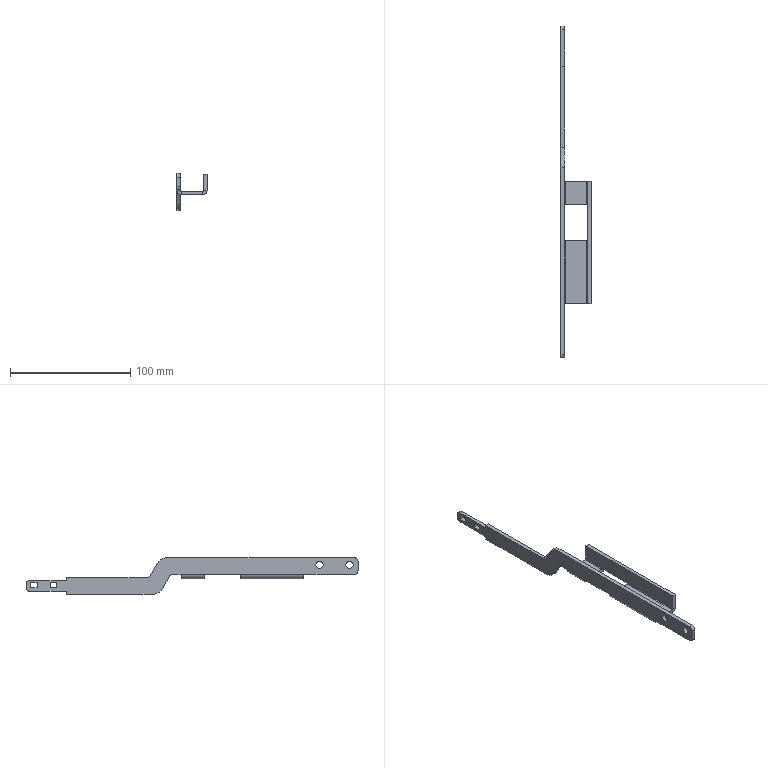Part | SolidWorks | features BaseBody 1 | 1 solid | 63 faces | box 25 x 276 x 30.5 mm | volume 20505 mm3 | plane 43 | cylinder 20 | commonest cylinder face diameters 6 x10 1 x4 7 x4 20 x2